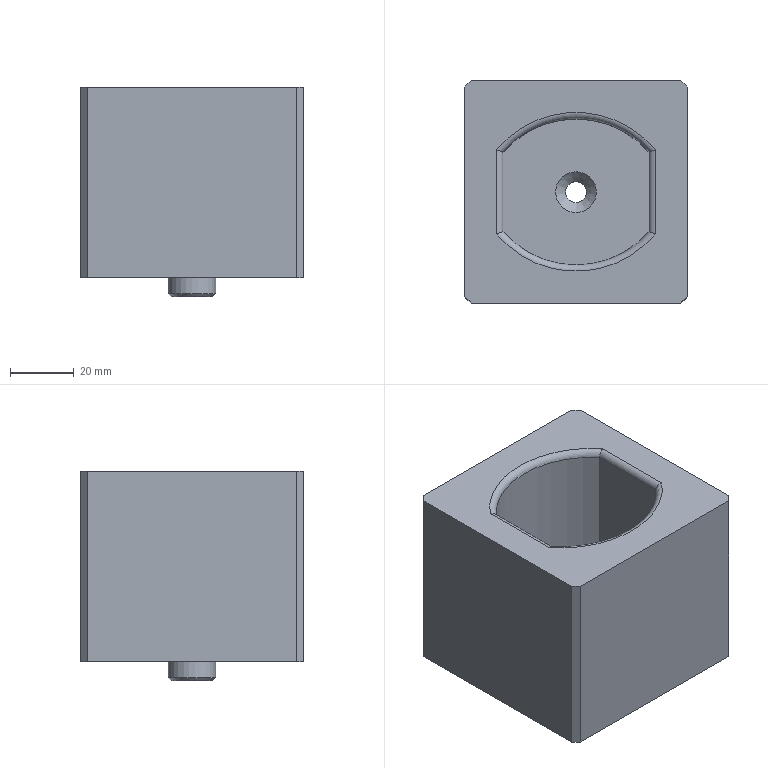Part | NX | 2 solids | 26 faces | box 70 x 70 x 66 mm | volume 193810 mm3 | plane 15 | cylinder 7 | cone 2 | torus 2 | commonest cylinder face diameters 4 x2 6.6 x2 60.881 x2 15 x1
STEP:
#1=CARTESIAN_POINT('',(0.,7.5,-65.));
#2=VERTEX_POINT('',#1);
#3=CARTESIAN_POINT('',(0.,0.,-65.));
#4=DIRECTION('',(0.,0.,-1.));
#5=DIRECTION('',(0.,1.,0.));
#6=AXIS2_PLACEMENT_3D('',#3,#4,#5);
#7=CIRCLE('',#6,7.5);
#8=EDGE_CURVE('',#2,#2,#7,.F.);
#9=ORIENTED_EDGE('',*,*,#8,.T.);
#10=EDGE_LOOP('',(#9));
#11=FACE_BOUND('',#10,.T.);
#12=CARTESIAN_POINT('',(0.,7.5,-60.));
#13=VERTEX_POINT('',#12);
#14=CARTESIAN_POINT('',(0.,0.,-60.));
#15=DIRECTION('',(0.,0.,-1.));
#16=DIRECTION('',(0.,1.,0.));
#17=AXIS2_PLACEMENT_3D('',#14,#15,#16);
#18=CIRCLE('',#17,7.5);
#19=EDGE_CURVE('',#13,#13,#18,.T.);
#20=ORIENTED_EDGE('',*,*,#19,.T.);
#21=EDGE_LOOP('',(#20));
#22=FACE_BOUND('',#21,.T.);
#23=CARTESIAN_POINT('',(0.,0.,-66.));
#24=DIRECTION('',(0.,0.,1.));
#25=DIRECTION('',(0.,-1.,0.));
#26=AXIS2_PLACEMENT_3D('',#23,#24,#25);
#27=CYLINDRICAL_SURFACE('',#26,7.5);
#28=ADVANCED_FACE('',(#11,#22),#27,.T.);
#29=CARTESIAN_POINT('',(0.,-3.3,-66.));
#30=VERTEX_POINT('',#29);
#31=CARTESIAN_POINT('',(0.,0.,-66.));
#32=DIRECTION('',(0.,0.,1.));
#33=DIRECTION('',(0.,-1.,0.));
#34=AXIS2_PLACEMENT_3D('',#31,#32,#33);
#35=CIRCLE('',#34,3.3);
#36=EDGE_CURVE('',#30,#30,#35,.T.);
#37=ORIENTED_EDGE('',*,*,#36,.T.);
#38=EDGE_LOOP('',(#37));
#39=FACE_BOUND('',#38,.T.);
#40=CARTESIAN_POINT('',(0.,6.5,-66.));
#41=VERTEX_POINT('',#40);
#42=CARTESIAN_POINT('',(0.,0.,-66.));
#43=DIRECTION('',(0.,0.,-1.));
#44=DIRECTION('',(0.,1.,0.));
#45=AXIS2_PLACEMENT_3D('',#42,#43,#44);
#46=CIRCLE('',#45,6.5);
#47=EDGE_CURVE('',#41,#41,#46,.T.);
#48=ORIENTED_EDGE('',*,*,#47,.T.);
#49=EDGE_LOOP('',(#48));
#50=FACE_BOUND('',#49,.T.);
#51=CARTESIAN_POINT('',(0.,0.,-66.));
#52=DIRECTION('',(0.,0.,-1.));
#53=DIRECTION('',(0.,1.,0.));
#54=AXIS2_PLACEMENT_3D('',#51,#52,#53);
#55=PLANE('',#54);
#56=ADVANCED_FACE('',(#39,#50),#55,.T.);
#57=CARTESIAN_POINT('',(0.,3.3,-60.));
#58=VERTEX_POINT('',#57);
#59=CARTESIAN_POINT('',(0.,0.,-60.));
#60=DIRECTION('',(0.,0.,-1.));
#61=DIRECTION('',(0.,1.,0.));
#62=AXIS2_PLACEMENT_3D('',#59,#60,#61);
#63=CIRCLE('',#62,3.3);
#64=EDGE_CURVE('',#58,#58,#63,.T.);
#65=ORIENTED_EDGE('',*,*,#64,.T.);
#66=EDGE_LOOP('',(#65));
#67=FACE_BOUND('',#66,.T.);
#68=ORIENTED_EDGE('',*,*,#19,.F.);
#69=EDGE_LOOP('',(#68));
#70=FACE_BOUND('',#69,.T.);
#71=CARTESIAN_POINT('',(0.,0.,-60.));
#72=DIRECTION('',(0.,0.,-1.));
#73=DIRECTION('',(0.,1.,0.));
#74=AXIS2_PLACEMENT_3D('',#71,#72,#73);
#75=PLANE('',#74);
#76=ADVANCED_FACE('',(#67,#70),#75,.F.);
#77=ORIENTED_EDGE('',*,*,#8,.F.);
#78=EDGE_LOOP('',(#77));
#79=FACE_BOUND('',#78,.T.);
#80=ORIENTED_EDGE('',*,*,#47,.F.);
#81=EDGE_LOOP('',(#80));
#82=FACE_BOUND('',#81,.T.);
#83=CARTESIAN_POINT('',(0.,0.,-66.));
#84=DIRECTION('',(0.,0.,1.));
#85=DIRECTION('',(0.,-1.,0.));
#86=AXIS2_PLACEMENT_3D('',#83,#84,#85);
#87=CONICAL_SURFACE('',#86,6.5,0.7854);
#88=ADVANCED_FACE('',(#79,#82),#87,.T.);
#89=ORIENTED_EDGE('',*,*,#36,.F.);
#90=EDGE_LOOP('',(#89));
#91=FACE_BOUND('',#90,.T.);
#92=ORIENTED_EDGE('',*,*,#64,.F.);
#93=EDGE_LOOP('',(#92));
#94=FACE_BOUND('',#93,.T.);
#95=CARTESIAN_POINT('',(0.,0.,-55.));
#96=DIRECTION('',(0.,0.,1.));
#97=DIRECTION('',(0.,-1.,0.));
#98=AXIS2_PLACEMENT_3D('',#95,#96,#97);
#99=CYLINDRICAL_SURFACE('',#98,3.3);
#100=ADVANCED_FACE('',(#91,#94),#99,.F.);
#101=CLOSED_SHELL('',(#28,#56,#76,#88,#100));
#102=MANIFOLD_SOLID_BREP('',#101);
#103=CARTESIAN_POINT('',(25.,-13.233,0.));
#104=VERTEX_POINT('',#103);
#105=CARTESIAN_POINT('',(-25.,-13.233,0.));
#106=VERTEX_POINT('',#105);
#107=CARTESIAN_POINT('',(0.,7.44,0.));
#108=DIRECTION('',(0.,0.,-1.));
#109=DIRECTION('',(0.,1.,0.));
#110=AXIS2_PLACEMENT_3D('',#107,#108,#109);
#111=CIRCLE('',#110,32.44);
#112=EDGE_CURVE('',#104,#106,#111,.T.);
#113=ORIENTED_EDGE('',*,*,#112,.T.);
#114=CARTESIAN_POINT('',(-25.,13.233,0.));
#115=VERTEX_POINT('',#114);
#116=CARTESIAN_POINT('',(-25.,12.5,0.));
#117=DIRECTION('',(0.,1.,0.));
#118=VECTOR('',#117,1000.);
#119=LINE('',#116,#118);
#120=EDGE_CURVE('',#106,#115,#119,.T.);
#121=ORIENTED_EDGE('',*,*,#120,.T.);
#122=CARTESIAN_POINT('',(25.,13.233,0.));
#123=VERTEX_POINT('',#122);
#124=CARTESIAN_POINT('',(0.,-7.44,0.));
#125=DIRECTION('',(0.,0.,-1.));
#126=DIRECTION('',(0.,1.,0.));
#127=AXIS2_PLACEMENT_3D('',#124,#125,#126);
#128=CIRCLE('',#127,32.44);
#129=EDGE_CURVE('',#115,#123,#128,.T.);
#130=ORIENTED_EDGE('',*,*,#129,.T.);
#131=CARTESIAN_POINT('',(25.,0.,0.));
#132=DIRECTION('',(0.,1.,0.));
#133=VECTOR('',#132,1000.);
#134=LINE('',#131,#133);
#135=EDGE_CURVE('',#123,#104,#134,.F.);
#136=ORIENTED_EDGE('',*,*,#135,.T.);
#137=EDGE_LOOP('',(#113,#121,#130,#136));
#138=FACE_BOUND('',#137,.T.);
#139=CARTESIAN_POINT('',(-33.,35.,0.));
#140=VERTEX_POINT('',#139);
#141=CARTESIAN_POINT('',(33.,35.,0.));
#142=VERTEX_POINT('',#141);
#143=CARTESIAN_POINT('',(-35.,35.,0.));
#144=DIRECTION('',(1.,0.,0.));
#145=VECTOR('',#144,1000.);
#146=LINE('',#143,#145);
#147=EDGE_CURVE('',#140,#142,#146,.T.);
#148=ORIENTED_EDGE('',*,*,#147,.F.);
#149=CARTESIAN_POINT('',(-35.,33.,0.));
#150=VERTEX_POINT('',#149);
#151=CARTESIAN_POINT('',(-35.,33.,0.));
#152=DIRECTION('',(0.7071,0.7071,0.));
#153=VECTOR('',#152,1000.);
#154=LINE('',#151,#153);
#155=EDGE_CURVE('',#140,#150,#154,.F.);
#156=ORIENTED_EDGE('',*,*,#155,.T.);
#157=CARTESIAN_POINT('',(-35.,-33.,0.));
#158=VERTEX_POINT('',#157);
#159=CARTESIAN_POINT('',(-35.,-35.,0.));
#160=DIRECTION('',(0.,1.,0.));
#161=VECTOR('',#160,1000.);
#162=LINE('',#159,#161);
#163=EDGE_CURVE('',#158,#150,#162,.T.);
#164=ORIENTED_EDGE('',*,*,#163,.F.);
#165=CARTESIAN_POINT('',(-33.,-35.,0.));
#166=VERTEX_POINT('',#165);
#167=CARTESIAN_POINT('',(-33.,-35.,0.));
#168=DIRECTION('',(0.7071,-0.7071,0.));
#169=VECTOR('',#168,1000.);
#170=LINE('',#167,#169);
#171=EDGE_CURVE('',#158,#166,#170,.T.);
#172=ORIENTED_EDGE('',*,*,#171,.T.);
#173=CARTESIAN_POINT('',(33.,-35.,0.));
#174=VERTEX_POINT('',#173);
#175=CARTESIAN_POINT('',(-35.,-35.,0.));
#176=DIRECTION('',(1.,0.,0.));
#177=VECTOR('',#176,1000.);
#178=LINE('',#175,#177);
#179=EDGE_CURVE('',#166,#174,#178,.T.);
#180=ORIENTED_EDGE('',*,*,#179,.T.);
#181=CARTESIAN_POINT('',(35.,-33.,0.));
#182=VERTEX_POINT('',#181);
#183=CARTESIAN_POINT('',(35.,-33.,0.));
#184=DIRECTION('',(-0.7071,-0.7071,0.));
#185=VECTOR('',#184,1000.);
#186=LINE('',#183,#185);
#187=EDGE_CURVE('',#174,#182,#186,.F.);
#188=ORIENTED_EDGE('',*,*,#187,.T.);
#189=CARTESIAN_POINT('',(35.,33.,0.));
#190=VERTEX_POINT('',#189);
#191=CARTESIAN_POINT('',(35.,-35.,0.));
#192=DIRECTION('',(0.,1.,0.));
#193=VECTOR('',#192,1000.);
#194=LINE('',#191,#193);
#195=EDGE_CURVE('',#182,#190,#194,.T.);
#196=ORIENTED_EDGE('',*,*,#195,.T.);
#197=CARTESIAN_POINT('',(33.,35.,0.));
#198=DIRECTION('',(-0.7071,0.7071,0.));
#199=VECTOR('',#198,1000.);
#200=LINE('',#197,#199);
#201=EDGE_CURVE('',#190,#142,#200,.T.);
#202=ORIENTED_EDGE('',*,*,#201,.T.);
#203=EDGE_LOOP('',(#148,#156,#164,#172,#180,#188,#196,#202));
#204=FACE_BOUND('',#203,.T.);
#205=CARTESIAN_POINT('',(0.,0.,0.));
#206=DIRECTION('',(0.,0.,-1.));
#207=DIRECTION('',(0.,1.,0.));
#208=AXIS2_PLACEMENT_3D('',#205,#206,#207);
#209=PLANE('',#208);
#210=ADVANCED_FACE('',(#138,#204),#209,.F.);
#211=ORIENTED_EDGE('',*,*,#163,.T.);
#212=CARTESIAN_POINT('',(-35.,33.,-60.));
#213=VERTEX_POINT('',#212);
#214=CARTESIAN_POINT('',(-35.,33.,0.));
#215=DIRECTION('',(0.,0.,-1.));
#216=VECTOR('',#215,1000.);
#217=LINE('',#214,#216);
#218=EDGE_CURVE('',#150,#213,#217,.T.);
#219=ORIENTED_EDGE('',*,*,#218,.T.);
#220=CARTESIAN_POINT('',(-35.,-33.,-60.));
#221=VERTEX_POINT('',#220);
#222=CARTESIAN_POINT('',(-35.,-35.,-60.));
#223=DIRECTION('',(0.,1.,0.));
#224=VECTOR('',#223,1000.);
#225=LINE('',#222,#224);
#226=EDGE_CURVE('',#221,#213,#225,.T.);
#227=ORIENTED_EDGE('',*,*,#226,.F.);
#228=CARTESIAN_POINT('',(-35.,-33.,0.));
#229=DIRECTION('',(0.,0.,1.));
#230=VECTOR('',#229,1000.);
#231=LINE('',#228,#230);
#232=EDGE_CURVE('',#221,#158,#231,.T.);
#233=ORIENTED_EDGE('',*,*,#232,.T.);
#234=EDGE_LOOP('',(#211,#219,#227,#233));
#235=FACE_BOUND('',#234,.T.);
#236=CARTESIAN_POINT('',(-35.,-35.,0.));
#237=DIRECTION('',(-1.,0.,0.));
#238=DIRECTION('',(0.,-1.,0.));
#239=AXIS2_PLACEMENT_3D('',#236,#237,#238);
#240=PLANE('',#239);
#241=ADVANCED_FACE('',(#235),#240,.T.);
#242=ORIENTED_EDGE('',*,*,#179,.F.);
#243=CARTESIAN_POINT('',(-33.,-35.,-60.));
#244=VERTEX_POINT('',#243);
#245=CARTESIAN_POINT('',(-33.,-35.,-60.));
#246=DIRECTION('',(0.,0.,-1.));
#247=VECTOR('',#246,1000.);
#248=LINE('',#245,#247);
#249=EDGE_CURVE('',#166,#244,#248,.T.);
#250=ORIENTED_EDGE('',*,*,#249,.T.);
#251=CARTESIAN_POINT('',(33.,-35.,-60.));
#252=VERTEX_POINT('',#251);
#253=CARTESIAN_POINT('',(-35.,-35.,-60.));
#254=DIRECTION('',(1.,0.,0.));
#255=VECTOR('',#254,1000.);
#256=LINE('',#253,#255);
#257=EDGE_CURVE('',#244,#252,#256,.T.);
#258=ORIENTED_EDGE('',*,*,#257,.T.);
#259=CARTESIAN_POINT('',(33.,-35.,0.));
#260=DIRECTION('',(0.,0.,1.));
#261=VECTOR('',#260,1000.);
#262=LINE('',#259,#261);
#263=EDGE_CURVE('',#252,#174,#262,.T.);
#264=ORIENTED_EDGE('',*,*,#263,.T.);
#265=EDGE_LOOP('',(#242,#250,#258,#264));
#266=FACE_BOUND('',#265,.T.);
#267=CARTESIAN_POINT('',(-35.,-35.,0.));
#268=DIRECTION('',(0.,1.,0.));
#269=DIRECTION('',(-1.,0.,0.));
#270=AXIS2_PLACEMENT_3D('',#267,#268,#269);
#271=PLANE('',#270);
#272=ADVANCED_FACE('',(#266),#271,.F.);
#273=ORIENTED_EDGE('',*,*,#195,.F.);
#274=CARTESIAN_POINT('',(35.,-33.,-60.));
#275=VERTEX_POINT('',#274);
#276=CARTESIAN_POINT('',(35.,-33.,0.));
#277=DIRECTION('',(0.,0.,-1.));
#278=VECTOR('',#277,1000.);
#279=LINE('',#276,#278);
#280=EDGE_CURVE('',#182,#275,#279,.T.);
#281=ORIENTED_EDGE('',*,*,#280,.T.);
#282=CARTESIAN_POINT('',(35.,33.,-60.));
#283=VERTEX_POINT('',#282);
#284=CARTESIAN_POINT('',(35.,-35.,-60.));
#285=DIRECTION('',(0.,1.,0.));
#286=VECTOR('',#285,1000.);
#287=LINE('',#284,#286);
#288=EDGE_CURVE('',#275,#283,#287,.T.);
#289=ORIENTED_EDGE('',*,*,#288,.T.);
#290=CARTESIAN_POINT('',(35.,33.,0.));
#291=DIRECTION('',(0.,0.,1.));
#292=VECTOR('',#291,1000.);
#293=LINE('',#290,#292);
#294=EDGE_CURVE('',#283,#190,#293,.T.);
#295=ORIENTED_EDGE('',*,*,#294,.T.);
#296=EDGE_LOOP('',(#273,#281,#289,#295));
#297=FACE_BOUND('',#296,.T.);
#298=CARTESIAN_POINT('',(35.,-35.,0.));
#299=DIRECTION('',(-1.,0.,0.));
#300=DIRECTION('',(0.,-1.,0.));
#301=AXIS2_PLACEMENT_3D('',#298,#299,#300);
#302=PLANE('',#301);
#303=ADVANCED_FACE('',(#297),#302,.F.);
#304=CARTESIAN_POINT('',(-33.,35.,-60.));
#305=VERTEX_POINT('',#304);
#306=CARTESIAN_POINT('',(33.,35.,-60.));
#307=VERTEX_POINT('',#306);
#308=CARTESIAN_POINT('',(-35.,35.,-60.));
#309=DIRECTION('',(1.,0.,0.));
#310=VECTOR('',#309,1000.);
#311=LINE('',#308,#310);
#312=EDGE_CURVE('',#305,#307,#311,.T.);
#313=ORIENTED_EDGE('',*,*,#312,.F.);
#314=CARTESIAN_POINT('',(-33.,35.,0.));
#315=DIRECTION('',(0.,0.,1.));
#316=VECTOR('',#315,1000.);
#317=LINE('',#314,#316);
#318=EDGE_CURVE('',#305,#140,#317,.T.);
#319=ORIENTED_EDGE('',*,*,#318,.T.);
#320=ORIENTED_EDGE('',*,*,#147,.T.);
#321=CARTESIAN_POINT('',(33.,35.,-60.));
#322=DIRECTION('',(0.,0.,-1.));
#323=VECTOR('',#322,1000.);
#324=LINE('',#321,#323);
#325=EDGE_CURVE('',#142,#307,#324,.T.);
#326=ORIENTED_EDGE('',*,*,#325,.T.);
#327=EDGE_LOOP('',(#313,#319,#320,#326));
#328=FACE_BOUND('',#327,.T.);
#329=CARTESIAN_POINT('',(-35.,35.,0.));
#330=DIRECTION('',(0.,1.,0.));
#331=DIRECTION('',(-1.,0.,0.));
#332=AXIS2_PLACEMENT_3D('',#329,#330,#331);
#333=PLANE('',#332);
#334=ADVANCED_FACE('',(#328),#333,.T.);
#335=CARTESIAN_POINT('',(0.,3.3,-60.));
#336=VERTEX_POINT('',#335);
#337=CARTESIAN_POINT('',(0.,0.,-60.));
#338=DIRECTION('',(0.,0.,-1.));
#339=DIRECTION('',(0.,1.,0.));
#340=AXIS2_PLACEMENT_3D('',#337,#338,#339);
#341=CIRCLE('',#340,3.3);
#342=EDGE_CURVE('',#336,#336,#341,.T.);
#343=ORIENTED_EDGE('',*,*,#342,.F.);
#344=EDGE_LOOP('',(#343));
#345=FACE_BOUND('',#344,.T.);
#346=ORIENTED_EDGE('',*,*,#226,.T.);
#347=CARTESIAN_POINT('',(-34.,34.,-60.));
#348=DIRECTION('',(-0.7071,-0.7071,0.));
#349=VECTOR('',#348,1000.);
#350=LINE('',#347,#349);
#351=EDGE_CURVE('',#213,#305,#350,.F.);
#352=ORIENTED_EDGE('',*,*,#351,.T.);
#353=ORIENTED_EDGE('',*,*,#312,.T.);
#354=CARTESIAN_POINT('',(34.,34.,-60.));
#355=DIRECTION('',(0.7071,-0.7071,0.));
#356=VECTOR('',#355,1000.);
#357=LINE('',#354,#356);
#358=EDGE_CURVE('',#307,#283,#357,.T.);
#359=ORIENTED_EDGE('',*,*,#358,.T.);
#360=ORIENTED_EDGE('',*,*,#288,.F.);
#361=CARTESIAN_POINT('',(34.,-34.,-60.));
#362=DIRECTION('',(0.7071,0.7071,0.));
#363=VECTOR('',#362,1000.);
#364=LINE('',#361,#363);
#365=EDGE_CURVE('',#275,#252,#364,.F.);
#366=ORIENTED_EDGE('',*,*,#365,.T.);
#367=ORIENTED_EDGE('',*,*,#257,.F.);
#368=CARTESIAN_POINT('',(-34.,-34.,-60.));
#369=DIRECTION('',(-0.7071,0.7071,0.));
#370=VECTOR('',#369,1000.);
#371=LINE('',#368,#370);
#372=EDGE_CURVE('',#244,#221,#371,.T.);
#373=ORIENTED_EDGE('',*,*,#372,.T.);
#374=EDGE_LOOP('',(#346,#352,#353,#359,#360,#366,#367,#373));
#375=FACE_BOUND('',#374,.T.);
#376=CARTESIAN_POINT('',(0.,0.,-60.));
#377=DIRECTION('',(0.,0.,-1.));
#378=DIRECTION('',(0.,1.,0.));
#379=AXIS2_PLACEMENT_3D('',#376,#377,#378);
#380=PLANE('',#379);
#381=ADVANCED_FACE('',(#345,#375),#380,.T.);
#382=CARTESIAN_POINT('',(-23.,12.5,-55.));
#383=VERTEX_POINT('',#382);
#384=CARTESIAN_POINT('',(-23.,12.5,-2.));
#385=VERTEX_POINT('',#384);
#386=CARTESIAN_POINT('',(-23.,12.5,-55.));
#387=DIRECTION('',(0.,0.,1.));
#388=VECTOR('',#387,1000.);
#389=LINE('',#386,#388);
#390=EDGE_CURVE('',#383,#385,#389,.T.);
#391=ORIENTED_EDGE('',*,*,#390,.T.);
#392=CARTESIAN_POINT('',(-23.,-12.5,-2.));
#393=VERTEX_POINT('',#392);
#394=CARTESIAN_POINT('',(-23.,-12.5,-2.));
#395=DIRECTION('',(0.,1.,0.));
#396=VECTOR('',#395,1000.);
#397=LINE('',#394,#396);
#398=EDGE_CURVE('',#385,#393,#397,.F.);
#399=ORIENTED_EDGE('',*,*,#398,.T.);
#400=CARTESIAN_POINT('',(-23.,-12.5,-55.));
#401=VERTEX_POINT('',#400);
#402=CARTESIAN_POINT('',(-23.,-12.5,-55.));
#403=DIRECTION('',(0.,0.,1.));
#404=VECTOR('',#403,1000.);
#405=LINE('',#402,#404);
#406=EDGE_CURVE('',#401,#393,#405,.T.);
#407=ORIENTED_EDGE('',*,*,#406,.F.);
#408=CARTESIAN_POINT('',(-23.,-12.5,-55.));
#409=DIRECTION('',(0.,1.,0.));
#410=VECTOR('',#409,1000.);
#411=LINE('',#408,#410);
#412=EDGE_CURVE('',#401,#383,#411,.T.);
#413=ORIENTED_EDGE('',*,*,#412,.T.);
#414=EDGE_LOOP('',(#391,#399,#407,#413));
#415=FACE_BOUND('',#414,.T.);
#416=CARTESIAN_POINT('',(-23.,-12.5,-55.));
#417=DIRECTION('',(1.,0.,0.));
#418=DIRECTION('',(0.,1.,0.));
#419=AXIS2_PLACEMENT_3D('',#416,#417,#418);
#420=PLANE('',#419);
#421=ADVANCED_FACE('',(#415),#420,.T.);
#422=CARTESIAN_POINT('',(23.,12.5,-55.));
#423=VERTEX_POINT('',#422);
#424=CARTESIAN_POINT('',(23.,12.5,-2.));
#425=VERTEX_POINT('',#424);
#426=CARTESIAN_POINT('',(23.,12.5,-55.));
#427=DIRECTION('',(0.,0.,1.));
#428=VECTOR('',#427,1000.);
#429=LINE('',#426,#428);
#430=EDGE_CURVE('',#423,#425,#429,.T.);
#431=ORIENTED_EDGE('',*,*,#430,.T.);
#432=CARTESIAN_POINT('',(0.,-7.44,-2.));
#433=DIRECTION('',(0.,0.,-1.));
#434=DIRECTION('',(0.,1.,0.));
#435=AXIS2_PLACEMENT_3D('',#432,#433,#434);
#436=CIRCLE('',#435,30.44);
#437=EDGE_CURVE('',#425,#385,#436,.F.);
#438=ORIENTED_EDGE('',*,*,#437,.T.);
#439=ORIENTED_EDGE('',*,*,#390,.F.);
#440=CARTESIAN_POINT('',(0.,-7.44,-55.));
#441=DIRECTION('',(0.,0.,-1.));
#442=DIRECTION('',(0.,1.,0.));
#443=AXIS2_PLACEMENT_3D('',#440,#441,#442);
#444=CIRCLE('',#443,30.44);
#445=EDGE_CURVE('',#383,#423,#444,.T.);
#446=ORIENTED_EDGE('',*,*,#445,.T.);
#447=EDGE_LOOP('',(#431,#438,#439,#446));
#448=FACE_BOUND('',#447,.T.);
#449=CARTESIAN_POINT('',(0.,-7.44,-55.));
#450=DIRECTION('',(0.,0.,1.));
#451=DIRECTION('',(0.,-1.,0.));
#452=AXIS2_PLACEMENT_3D('',#449,#450,#451);
#453=CYLINDRICAL_SURFACE('',#452,30.44);
#454=ADVANCED_FACE('',(#448),#453,.F.);
#455=CARTESIAN_POINT('',(23.,-12.5,-55.));
#456=VERTEX_POINT('',#455);
#457=CARTESIAN_POINT('',(23.,-12.5,-2.));
#458=VERTEX_POINT('',#457);
#459=CARTESIAN_POINT('',(23.,-12.5,-55.));
#460=DIRECTION('',(0.,0.,1.));
#461=VECTOR('',#460,1000.);
#462=LINE('',#459,#461);
#463=EDGE_CURVE('',#456,#458,#462,.T.);
#464=ORIENTED_EDGE('',*,*,#463,.T.);
#465=CARTESIAN_POINT('',(23.,-12.5,-2.));
#466=DIRECTION('',(0.,1.,0.));
#467=VECTOR('',#466,1000.);
#468=LINE('',#465,#467);
#469=EDGE_CURVE('',#458,#425,#468,.T.);
#470=ORIENTED_EDGE('',*,*,#469,.T.);
#471=ORIENTED_EDGE('',*,*,#430,.F.);
#472=CARTESIAN_POINT('',(23.,-12.5,-55.));
#473=DIRECTION('',(0.,1.,0.));
#474=VECTOR('',#473,1000.);
#475=LINE('',#472,#474);
#476=EDGE_CURVE('',#456,#423,#475,.T.);
#477=ORIENTED_EDGE('',*,*,#476,.F.);
#478=EDGE_LOOP('',(#464,#470,#471,#477));
#479=FACE_BOUND('',#478,.T.);
#480=CARTESIAN_POINT('',(23.,-12.5,-55.));
#481=DIRECTION('',(1.,0.,0.));
#482=DIRECTION('',(0.,1.,0.));
#483=AXIS2_PLACEMENT_3D('',#480,#481,#482);
#484=PLANE('',#483);
#485=ADVANCED_FACE('',(#479),#484,.F.);
#486=ORIENTED_EDGE('',*,*,#406,.T.);
#487=CARTESIAN_POINT('',(0.,7.44,-2.));
#488=DIRECTION('',(0.,0.,-1.));
#489=DIRECTION('',(0.,1.,0.));
#490=AXIS2_PLACEMENT_3D('',#487,#488,#489);
#491=CIRCLE('',#490,30.44);
#492=EDGE_CURVE('',#393,#458,#491,.F.);
#493=ORIENTED_EDGE('',*,*,#492,.T.);
#494=ORIENTED_EDGE('',*,*,#463,.F.);
#495=CARTESIAN_POINT('',(0.,7.44,-55.));
#496=DIRECTION('',(0.,0.,1.));
#497=DIRECTION('',(0.,-1.,0.));
#498=AXIS2_PLACEMENT_3D('',#495,#496,#497);
#499=CIRCLE('',#498,30.44);
#500=EDGE_CURVE('',#401,#456,#499,.T.);
#501=ORIENTED_EDGE('',*,*,#500,.F.);
#502=EDGE_LOOP('',(#486,#493,#494,#501));
#503=FACE_BOUND('',#502,.T.);
#504=CARTESIAN_POINT('',(0.,7.44,-55.));
#505=DIRECTION('',(0.,0.,1.));
#506=DIRECTION('',(0.,-1.,0.));
#507=AXIS2_PLACEMENT_3D('',#504,#505,#506);
#508=CYLINDRICAL_SURFACE('',#507,30.44);
#509=ADVANCED_FACE('',(#503),#508,.F.);
#510=CARTESIAN_POINT('',(0.,-6.4,-55.));
#511=VERTEX_POINT('',#510);
#512=CARTESIAN_POINT('',(0.,0.,-55.));
#513=DIRECTION('',(0.,0.,1.));
#514=DIRECTION('',(0.,-1.,0.));
#515=AXIS2_PLACEMENT_3D('',#512,#513,#514);
#516=CIRCLE('',#515,6.4);
#517=EDGE_CURVE('',#511,#511,#516,.T.);
#518=ORIENTED_EDGE('',*,*,#517,.F.);
#519=EDGE_LOOP('',(#518));
#520=FACE_BOUND('',#519,.T.);
#521=ORIENTED_EDGE('',*,*,#412,.F.);
#522=ORIENTED_EDGE('',*,*,#500,.T.);
#523=ORIENTED_EDGE('',*,*,#476,.T.);
#524=ORIENTED_EDGE('',*,*,#445,.F.);
#525=EDGE_LOOP('',(#521,#522,#523,#524));
#526=FACE_BOUND('',#525,.T.);
#527=CARTESIAN_POINT('',(0.,-7.44,-55.));
#528=DIRECTION('',(0.,0.,-1.));
#529=DIRECTION('',(0.,1.,0.));
#530=AXIS2_PLACEMENT_3D('',#527,#528,#529);
#531=PLANE('',#530);
#532=ADVANCED_FACE('',(#520,#526),#531,.F.);
#533=CARTESIAN_POINT('',(23.,12.5,-2.));
#534=CARTESIAN_POINT('',(23.,12.5,-1.454));
#535=CARTESIAN_POINT('',(23.468,12.675,-0.4021));
#536=CARTESIAN_POINT('',(24.494,13.051,0.));
#537=CARTESIAN_POINT('',(25.,13.233,0.));
#538=B_SPLINE_CURVE_WITH_KNOTS('',3,(#533,#534,#535,#536,#537),.UNSPECIFIED.,.F.,.F.,(4,1,4),(0.,0.001613,0.003226),.UNSPECIFIED.);
#539=EDGE_CURVE('',#425,#123,#538,.T.);
#540=ORIENTED_EDGE('',*,*,#539,.F.);
#541=ORIENTED_EDGE('',*,*,#469,.F.);
#542=CARTESIAN_POINT('',(23.,-12.5,-2.));
#543=CARTESIAN_POINT('',(23.,-12.5,-1.454));
#544=CARTESIAN_POINT('',(23.468,-12.675,-0.4021));
#545=CARTESIAN_POINT('',(24.494,-13.051,0.));
#546=CARTESIAN_POINT('',(25.,-13.233,0.));
#547=B_SPLINE_CURVE_WITH_KNOTS('',3,(#542,#543,#544,#545,#546),.UNSPECIFIED.,.F.,.F.,(4,1,4),(0.,0.001613,0.003226),.UNSPECIFIED.);
#548=EDGE_CURVE('',#104,#458,#547,.F.);
#549=ORIENTED_EDGE('',*,*,#548,.F.);
#550=ORIENTED_EDGE('',*,*,#135,.F.);
#551=EDGE_LOOP('',(#540,#541,#549,#550));
#552=FACE_BOUND('',#551,.T.);
#553=CARTESIAN_POINT('',(25.,-12.5,-2.));
#554=DIRECTION('',(0.,1.,0.));
#555=DIRECTION('',(-1.,0.,0.));
#556=AXIS2_PLACEMENT_3D('',#553,#554,#555);
#557=CYLINDRICAL_SURFACE('',#556,2.);
#558=ADVANCED_FACE('',(#552),#557,.T.);
#559=ORIENTED_EDGE('',*,*,#548,.T.);
#560=ORIENTED_EDGE('',*,*,#492,.F.);
#561=CARTESIAN_POINT('',(-23.,-12.5,-2.));
#562=CARTESIAN_POINT('',(-23.,-12.5,-1.454));
#563=CARTESIAN_POINT('',(-23.468,-12.675,-0.4021));
#564=CARTESIAN_POINT('',(-24.494,-13.051,0.));
#565=CARTESIAN_POINT('',(-25.,-13.233,0.));
#566=B_SPLINE_CURVE_WITH_KNOTS('',3,(#561,#562,#563,#564,#565),.UNSPECIFIED.,.F.,.F.,(4,1,4),(0.,0.001613,0.003226),.UNSPECIFIED.);
#567=EDGE_CURVE('',#106,#393,#566,.F.);
#568=ORIENTED_EDGE('',*,*,#567,.F.);
#569=ORIENTED_EDGE('',*,*,#112,.F.);
#570=EDGE_LOOP('',(#559,#560,#568,#569));
#571=FACE_BOUND('',#570,.T.);
#572=CARTESIAN_POINT('',(0.,7.44,-2.));
#573=DIRECTION('',(0.,0.,-1.));
#574=DIRECTION('',(0.,1.,0.));
#575=AXIS2_PLACEMENT_3D('',#572,#573,#574);
#576=TOROIDAL_SURFACE('',#575,32.44,2.);
#577=ADVANCED_FACE('',(#571),#576,.T.);
#578=ORIENTED_EDGE('',*,*,#539,.T.);
#579=ORIENTED_EDGE('',*,*,#129,.F.);
#580=CARTESIAN_POINT('',(-23.,12.5,-2.));
#581=CARTESIAN_POINT('',(-23.,12.5,-1.454));
#582=CARTESIAN_POINT('',(-23.468,12.675,-0.4021));
#583=CARTESIAN_POINT('',(-24.494,13.051,0.));
#584=CARTESIAN_POINT('',(-25.,13.233,0.));
#585=B_SPLINE_CURVE_WITH_KNOTS('',3,(#580,#581,#582,#583,#584),.UNSPECIFIED.,.F.,.F.,(4,1,4),(0.,0.001613,0.003226),.UNSPECIFIED.);
#586=EDGE_CURVE('',#385,#115,#585,.T.);
#587=ORIENTED_EDGE('',*,*,#586,.F.);
#588=ORIENTED_EDGE('',*,*,#437,.F.);
#589=EDGE_LOOP('',(#578,#579,#587,#588));
#590=FACE_BOUND('',#589,.T.);
#591=CARTESIAN_POINT('',(0.,-7.44,-2.));
#592=DIRECTION('',(0.,0.,-1.));
#593=DIRECTION('',(0.,1.,0.));
#594=AXIS2_PLACEMENT_3D('',#591,#592,#593);
#595=TOROIDAL_SURFACE('',#594,32.44,2.);
#596=ADVANCED_FACE('',(#590),#595,.T.);
#597=ORIENTED_EDGE('',*,*,#567,.T.);
#598=ORIENTED_EDGE('',*,*,#398,.F.);
#599=ORIENTED_EDGE('',*,*,#586,.T.);
#600=ORIENTED_EDGE('',*,*,#120,.F.);
#601=EDGE_LOOP('',(#597,#598,#599,#600));
#602=FACE_BOUND('',#601,.T.);
#603=CARTESIAN_POINT('',(-25.,0.,-2.));
#604=DIRECTION('',(0.,-1.,0.));
#605=DIRECTION('',(1.,0.,0.));
#606=AXIS2_PLACEMENT_3D('',#603,#604,#605);
#607=CYLINDRICAL_SURFACE('',#606,2.);
#608=ADVANCED_FACE('',(#602),#607,.T.);
#609=ORIENTED_EDGE('',*,*,#155,.F.);
#610=ORIENTED_EDGE('',*,*,#318,.F.);
#611=ORIENTED_EDGE('',*,*,#351,.F.);
#612=ORIENTED_EDGE('',*,*,#218,.F.);
#613=EDGE_LOOP('',(#609,#610,#611,#612));
#614=FACE_BOUND('',#613,.T.);
#615=CARTESIAN_POINT('',(-35.,33.,0.));
#616=DIRECTION('',(0.7071,-0.7071,0.));
#617=DIRECTION('',(0.,0.,-1.));
#618=AXIS2_PLACEMENT_3D('',#615,#616,#617);
#619=PLANE('',#618);
#620=ADVANCED_FACE('',(#614),#619,.F.);
#621=ORIENTED_EDGE('',*,*,#171,.F.);
#622=ORIENTED_EDGE('',*,*,#232,.F.);
#623=ORIENTED_EDGE('',*,*,#372,.F.);
#624=ORIENTED_EDGE('',*,*,#249,.F.);
#625=EDGE_LOOP('',(#621,#622,#623,#624));
#626=FACE_BOUND('',#625,.T.);
#627=CARTESIAN_POINT('',(-33.,-35.,0.));
#628=DIRECTION('',(-0.7071,-0.7071,0.));
#629=DIRECTION('',(0.,0.,1.));
#630=AXIS2_PLACEMENT_3D('',#627,#628,#629);
#631=PLANE('',#630);
#632=ADVANCED_FACE('',(#626),#631,.T.);
#633=ORIENTED_EDGE('',*,*,#187,.F.);
#634=ORIENTED_EDGE('',*,*,#263,.F.);
#635=ORIENTED_EDGE('',*,*,#365,.F.);
#636=ORIENTED_EDGE('',*,*,#280,.F.);
#637=EDGE_LOOP('',(#633,#634,#635,#636));
#638=FACE_BOUND('',#637,.T.);
#639=CARTESIAN_POINT('',(35.,-33.,0.));
#640=DIRECTION('',(-0.7071,0.7071,0.));
#641=DIRECTION('',(0.,0.,-1.));
#642=AXIS2_PLACEMENT_3D('',#639,#640,#641);
#643=PLANE('',#642);
#644=ADVANCED_FACE('',(#638),#643,.F.);
#645=ORIENTED_EDGE('',*,*,#201,.F.);
#646=ORIENTED_EDGE('',*,*,#294,.F.);
#647=ORIENTED_EDGE('',*,*,#358,.F.);
#648=ORIENTED_EDGE('',*,*,#325,.F.);
#649=EDGE_LOOP('',(#645,#646,#647,#648));
#650=FACE_BOUND('',#649,.T.);
#651=CARTESIAN_POINT('',(33.,35.,0.));
#652=DIRECTION('',(0.7071,0.7071,0.));
#653=DIRECTION('',(0.,0.,1.));
#654=AXIS2_PLACEMENT_3D('',#651,#652,#653);
#655=PLANE('',#654);
#656=ADVANCED_FACE('',(#650),#655,.T.);
#657=ORIENTED_EDGE('',*,*,#342,.T.);
#658=EDGE_LOOP('',(#657));
#659=FACE_BOUND('',#658,.T.);
#660=CARTESIAN_POINT('',(0.,-3.3,-58.1));
#661=VERTEX_POINT('',#660);
#662=CARTESIAN_POINT('',(0.,0.,-58.1));
#663=DIRECTION('',(0.,0.,1.));
#664=DIRECTION('',(0.,-1.,0.));
#665=AXIS2_PLACEMENT_3D('',#662,#663,#664);
#666=CIRCLE('',#665,3.3);
#667=EDGE_CURVE('',#661,#661,#666,.T.);
#668=ORIENTED_EDGE('',*,*,#667,.T.);
#669=EDGE_LOOP('',(#668));
#670=FACE_BOUND('',#669,.T.);
#671=CARTESIAN_POINT('',(0.,0.,-55.));
#672=DIRECTION('',(0.,0.,1.));
#673=DIRECTION('',(0.,-1.,0.));
#674=AXIS2_PLACEMENT_3D('',#671,#672,#673);
#675=CYLINDRICAL_SURFACE('',#674,3.3);
#676=ADVANCED_FACE('',(#659,#670),#675,.F.);
#677=ORIENTED_EDGE('',*,*,#667,.F.);
#678=EDGE_LOOP('',(#677));
#679=FACE_BOUND('',#678,.T.);
#680=ORIENTED_EDGE('',*,*,#517,.T.);
#681=EDGE_LOOP('',(#680));
#682=FACE_BOUND('',#681,.T.);
#683=CARTESIAN_POINT('',(0.,0.,-55.));
#684=DIRECTION('',(0.,0.,1.));
#685=DIRECTION('',(0.,-1.,0.));
#686=AXIS2_PLACEMENT_3D('',#683,#684,#685);
#687=CONICAL_SURFACE('',#686,6.4,0.7854);
#688=ADVANCED_FACE('',(#679,#682),#687,.F.);
#689=CLOSED_SHELL('',(#210,#241,#272,#303,#334,#381,#421,#454,#485,#509,#532,#558,#577,#596,#608,#620,#632,#644,#656,#676,#688));
#690=MANIFOLD_SOLID_BREP('',#689);
#691=(LENGTH_UNIT()NAMED_UNIT(*)SI_UNIT(.MILLI.,.METRE.));
#692=UNCERTAINTY_MEASURE_WITH_UNIT(LENGTH_MEASURE(0.0508),#691,'','');
#693=(NAMED_UNIT(*)PLANE_ANGLE_UNIT()SI_UNIT($,.RADIAN.));
#694=(NAMED_UNIT(*)SI_UNIT($,.STERADIAN.)SOLID_ANGLE_UNIT());
#695=(GEOMETRIC_REPRESENTATION_CONTEXT(3)GLOBAL_UNCERTAINTY_ASSIGNED_CONTEXT((#692))GLOBAL_UNIT_ASSIGNED_CONTEXT((#691,#693,#694))REPRESENTATION_CONTEXT('',''));
#696=ADVANCED_BREP_SHAPE_REPRESENTATION('',(#102,#690),#695);